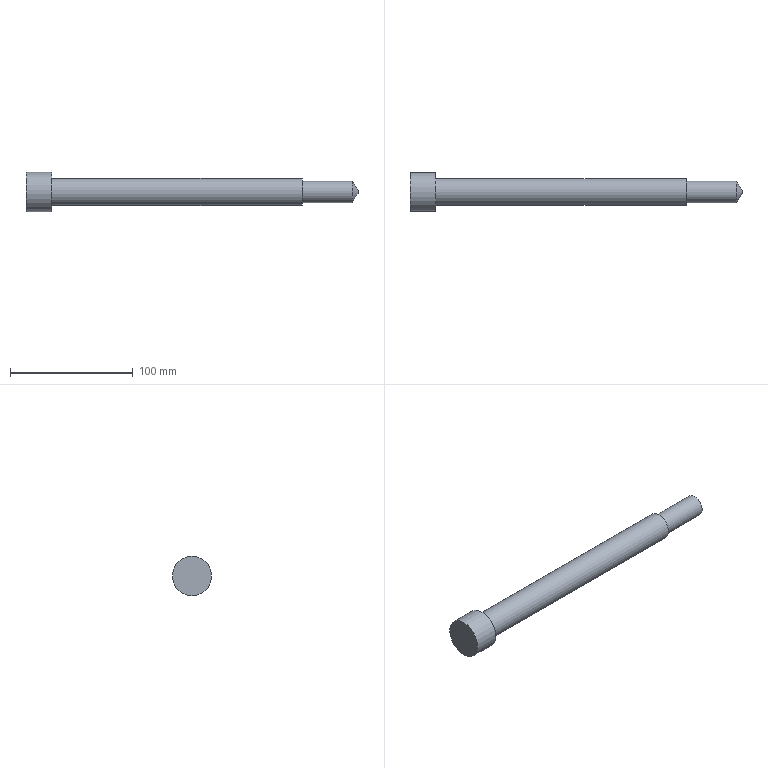Part | STEP file | solid 145 | 1 solid | 8 faces | box 270.5 x 32 x 32 mm | volume 104702 mm3 | plane 4 | cylinder 3 | cone 1 | commonest cylinder face diameters 17.5 x1 22 x1 32 x1